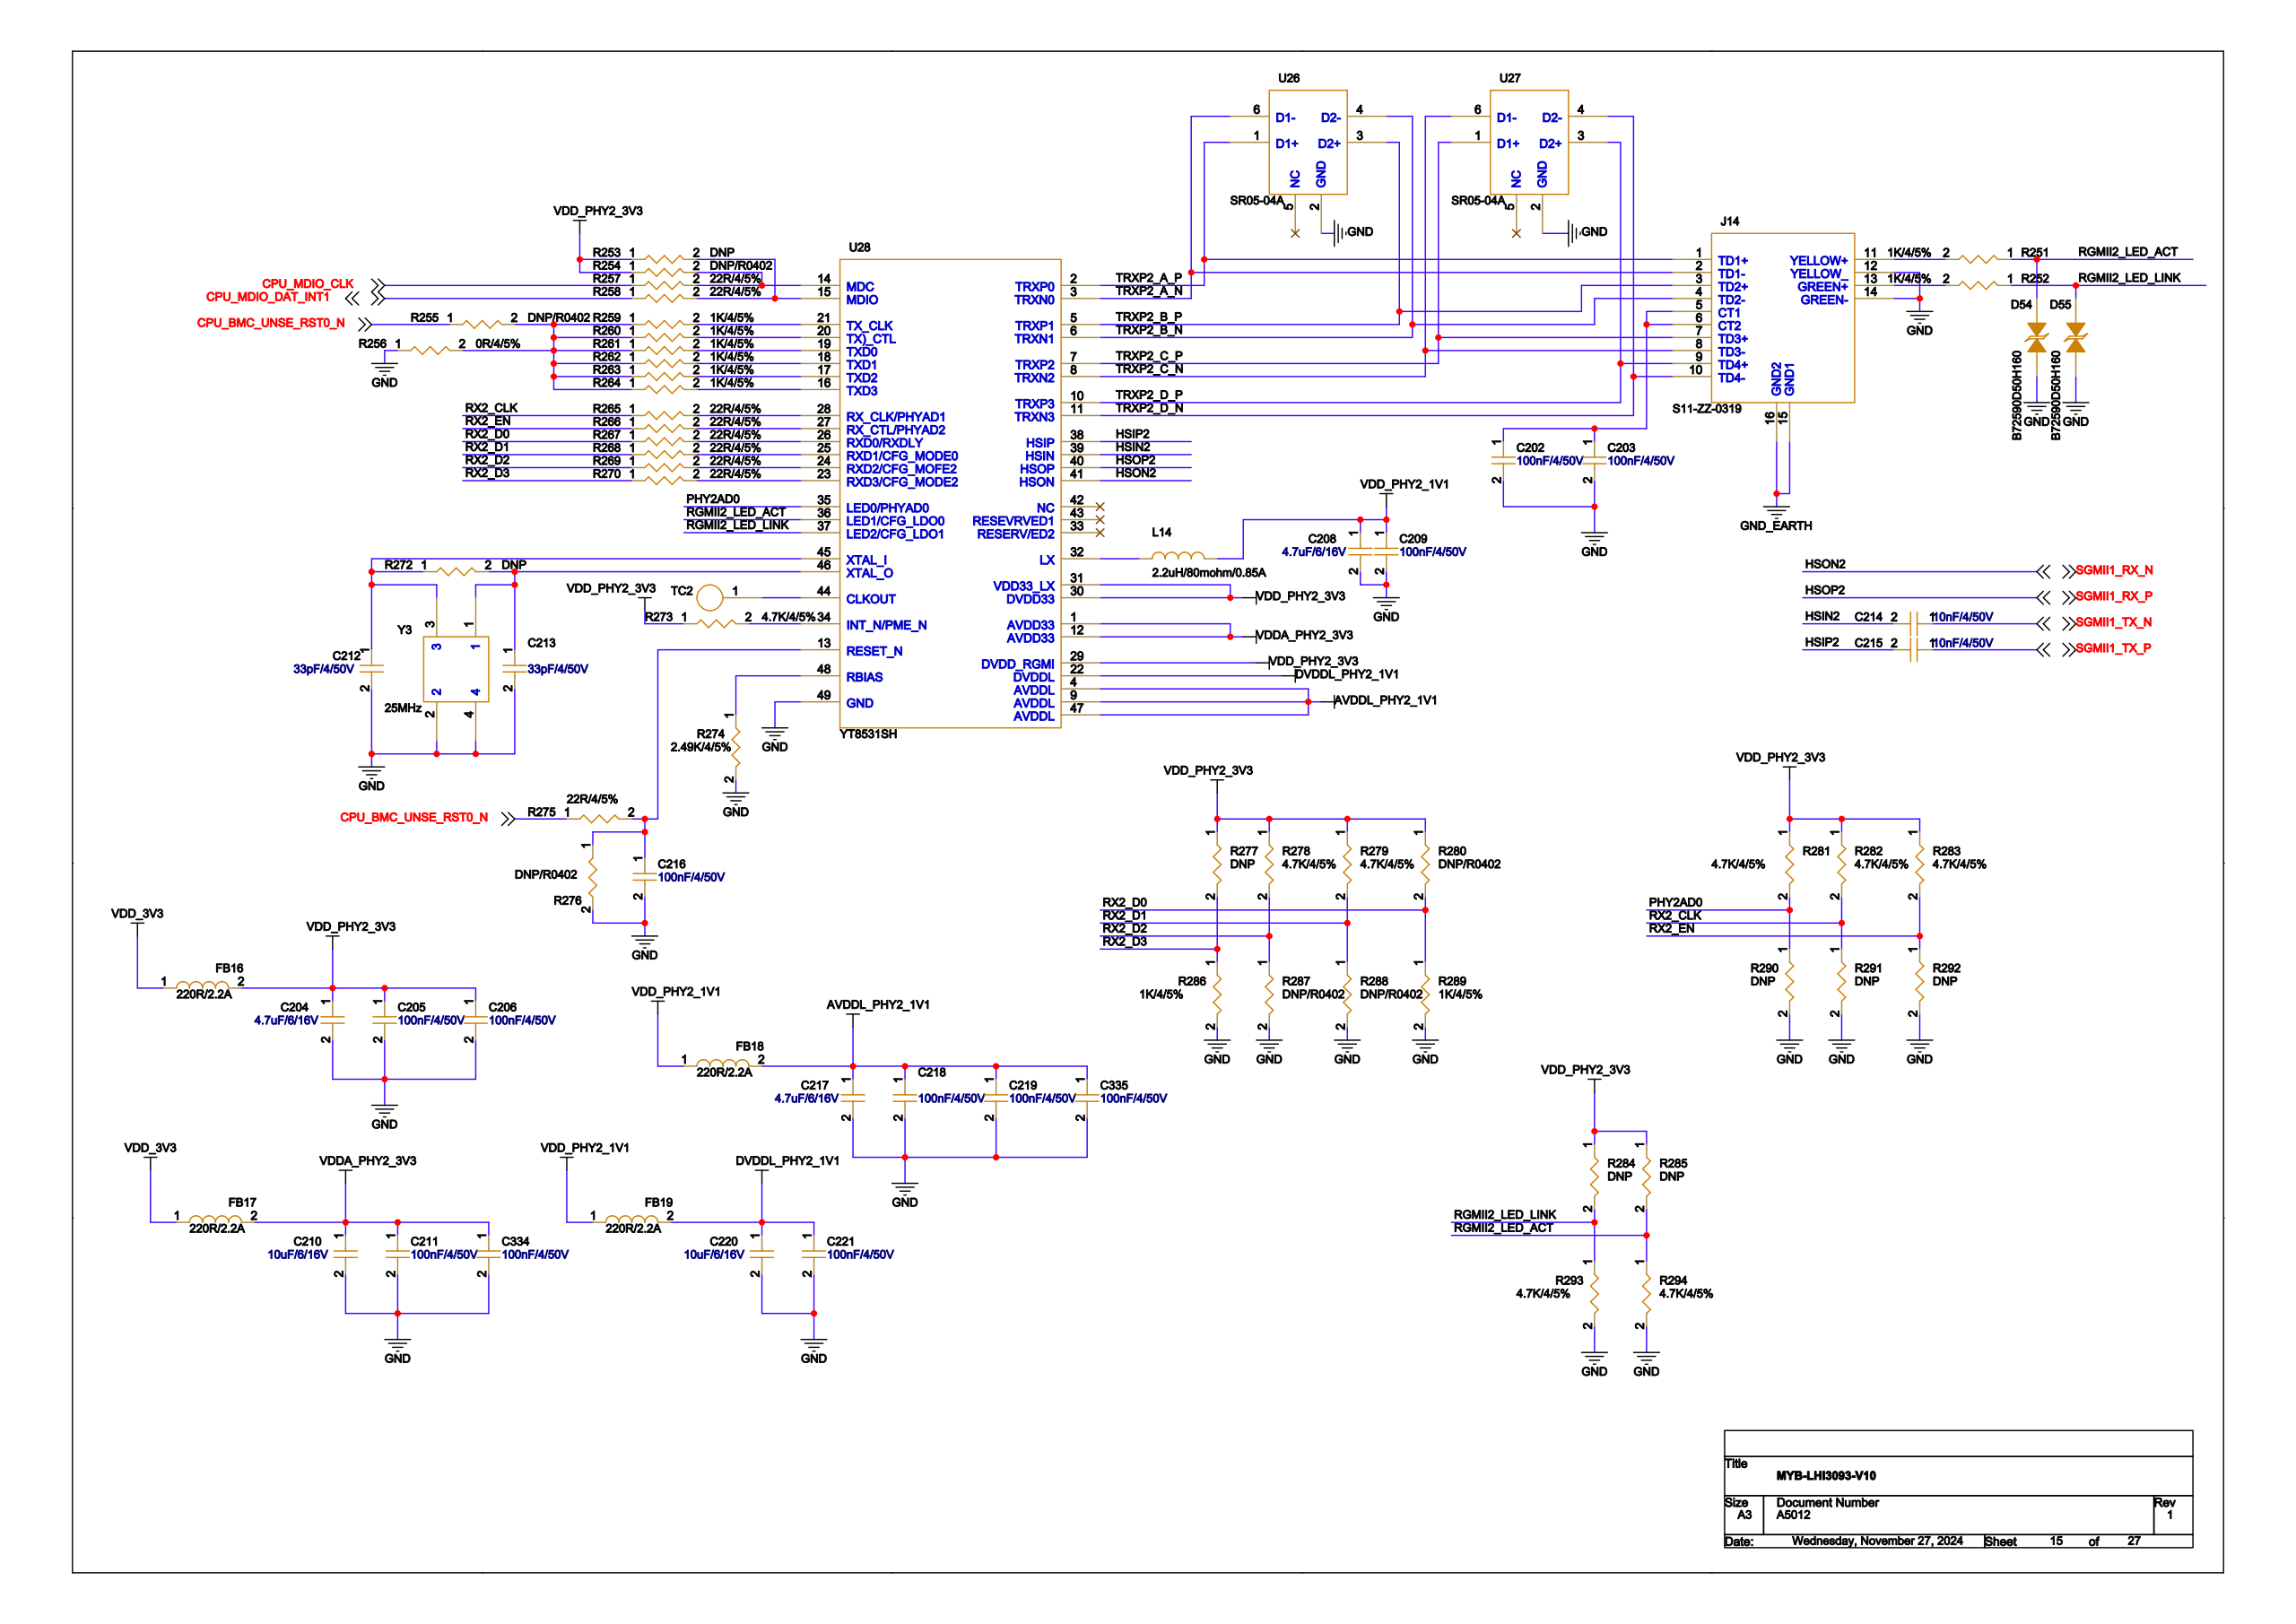Circuit board | Cadence Allegro | 1159 parts | 708 nets | one sheet of the schematic
Parts on this sheet (reference | value | footprint):
C202 | 100nF/4/50V | C0402
C203 | 100nF/4/50V | C0402
C204 | 4.7uF/6/16V | C0603
C205 | 100nF/4/50V | C0402
C206 | 100nF/4/50V | C0402
C208 | 4.7uF/6/16V | C0603
C209 | 100nF/4/50V | C0402
C210 | 10uF/6/16V | C0603
C211 | 100nF/4/50V | C0402
C212 | 33pF/4/50V | C0402
C213 | 33pF/4/50V | C0402
C214 | 10nF/4/50V | C0402
C215 | 10nF/4/50V | C0402
C216 | 100nF/4/50V | C0402
C217 | 4.7uF/6/16V | C0603
C218 | 100nF/4/50V | C0402
C219 | 100nF/4/50V | C0402
C220 | 10uF/6/16V | C0603
C221 | 100nF/4/50V | C0402
C334 | 100nF/4/50V | C0402
C335 | 100nF/4/50V | C0402
FB16 | 220R/2.2A | FB0603
FB17 | 220R/2.2A | FB0603
FB18 | 220R/2.2A | FB0603
FB19 | 220R/2.2A | FB0603
J14 | S11-ZZ-0319 | S11-ZZ-0319
L14 | 2.2uH/80mohm/0.85A | L2X2_5
R251 | 1K/4/5% | R0402
R252 | 1K/4/5% | R0402
R253 | DNP | R0402
R254 | DNP/R0402 | R0402
R255 | DNP/R0402 | R0402
R256 | 0R/4/5% | R0402
R257 | 22R/4/5% | R0402
R258 | 22R/4/5% | R0402
R259 | 1K/4/5% | R0402
R260 | 1K/4/5% | R0402
R261 | 1K/4/5% | R0402
R262 | 1K/4/5% | R0402
R263 | 1K/4/5% | R0402
R264 | 1K/4/5% | R0402
R265 | 22R/4/5% | R0402
R266 | 22R/4/5% | R0402
R267 | 22R/4/5% | R0402
R268 | 22R/4/5% | R0402
R269 | 22R/4/5% | R0402
R270 | 22R/4/5% | R0402
R272 | DNP | R0402
R273 | 4.7K/4/5% | R0402
R274 | 2.49K/4/5% | R0402
R275 | 22R/4/5% | R0402
R276 | DNP/R0402 | R0402
R277 | DNP | R0402
R278 | 4.7K/4/5% | R0402
R279 | 4.7K/4/5% | R0402
R280 | DNP/R0402 | R0402
R281 | 4.7K/4/5% | R0402
R282 | 4.7K/4/5% | R0402
R283 | 4.7K/4/5% | R0402
R284 | DNP | R0402
R285 | DNP | R0402
R286 | 1K/4/5% | R0402
R287 | DNP/R0402 | R0402
R288 | DNP/R0402 | R0402
R289 | 1K/4/5% | R0402
R290 | DNP | R0402
R291 | DNP | R0402
R292 | DNP | R0402
R293 | 4.7K/4/5% | R0402
R294 | 4.7K/4/5% | R0402
TC2 | TP | TP_SMT
U26 | SR05-04A | SOT23-6
U27 | SR05-04A | SOT23-6
U28 | YT8531SH | QFN48-0_4
Y3 | 25MHz | 3225
Nets of these parts (net: part-pin ...):
GND: C202-2 C203-2 C204-2 C205-2 C206-2 C208-2 C209-2 C210-2 C211-2 C212-2 C213-2 C216-2 C217-2 C218-2 C219-2 C220-2 C221-2 C334-2 C335-2 J14-12 J14-14 R256-1 R274-2 R276-2 R286-2 R287-2 R288-2 R289-2 R290-2 R291-2 R292-2 R293-2 R294-2 U26-2 U27-2 Y3-2 Y3-4 U28-49
VDD_3V3: FB16-1 FB17-1
N14989852: C202-1 C203-1 J14-5 J14-6
VDD_PHY2_3V3: C204-1 C205-1 C206-1 FB16-2 R253-1 R254-1 R273-1 R277-1 R278-1 R279-1 R280-1 R281-1 R282-1 R283-1 R284-1 R285-1 U28-29 U28-30 U28-31
VDD_PHY2_1V1: C208-1 C209-1 FB18-1 FB19-1 L14-2
VDDA_PHY2_3V3: C210-1 C211-1 C334-1 FB17-2 U28-1 U28-12
N14989098: C216-1 R275-2 R276-1 U28-13
AVDDL_PHY2_1V1: C217-1 C218-1 C219-1 C335-1 FB18-2 U28-4 U28-9 U28-47
DVDDL_PHY2_1V1: C220-1 C221-1 FB19-2 U28-22
GND_EARTH: J14-15 J14-16
N14988894: C212-1 R272-1 Y3-3 U28-45
N14988806: C213-1 R272-2 Y3-1 U28-46
SGMII1_TX_N: C214-1
HSIN2: C214-2 U28-39
SGMII1_TX_P: C215-1
HSIP2: C215-2 U28-38
RGMII2_LED_ACT: R251-1 R285-2 R294-1 U28-36
RGMII2_LED_LINK: R252-1 R284-2 R293-1 U28-37
N14989974: J14-13 R252-2
TRXP2_A_P: J14-1 U26-1 U28-2
TRXP2_A_N: J14-2 U26-6 U28-3
TRXP2_B_P: J14-3 U26-3 U28-5
TRXP2_B_N: J14-4 U26-4 U28-6
TRXP2_C_P: J14-7 U27-1 U28-7
TRXP2_C_N: J14-8 U27-6 U28-8
TRXP2_D_P: J14-9 U27-3 U28-10
TRXP2_D_N: J14-10 U27-4 U28-11
N14989970: J14-11 R251-2
N14988636: R255-2 R256-2 R259-1 R260-1 R261-1 R262-1 R263-1 R264-1
N14988500: R259-2 U28-21
N14988504: R260-2 U28-20
N14988508: R261-2 U28-19
N14988512: R262-2 U28-18
N14988528: R263-2 U28-17
N14988532: R264-2 U28-16
RX2_D3: R270-1 R277-2 R286-1
RX2_D0: R267-1 R280-2 R289-1
CPU_MDIO_CLK: R257-1
CPU_MDIO_DAT_INT1: R258-1
CPU_BMC_UNSE_RST0_N: R255-1 R275-1
N14988388: R254-2 R257-2 U28-14
N14988392: R253-2 R258-2 U28-15
RX2_CLK: R265-1 R282-2 R291-1
N14988536: R265-2 U28-28
RX2_EN: R266-1 R283-2 R292-1
N14988540: R266-2 U28-27
N14988552: R267-2 U28-26
RX2_D1: R268-1 R279-2 R288-1
N14988556: R268-2 U28-25
RX2_D2: R269-1 R278-2 R287-1
N14988560: R269-2 U28-24
N14988564: R270-2 U28-23
N14989030: R273-2 U28-34
PHY2AD0: R281-2 R290-1 U28-35
N14989058: R274-1 U28-48
N14988998: TC2-1 U28-44
SGMII1_RX_N: U28-41
SGMII1_RX_P: U28-40
N14989556: L14-1 U28-32